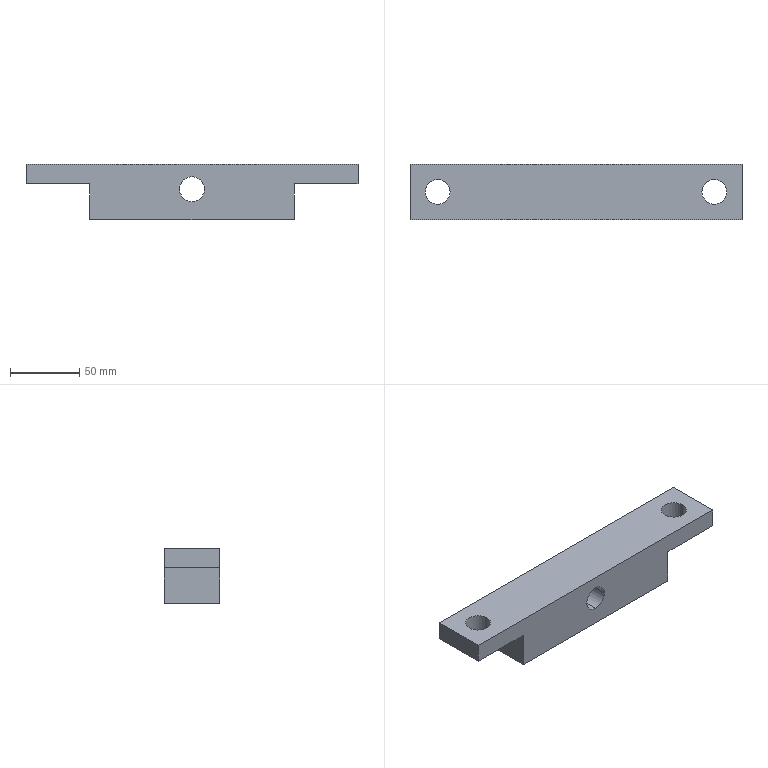Part | SolidWorks | features BaseBody 1 | 1 solid | 16 faces | box 240 x 40 x 40 mm | volume 271016 mm3 | plane 10 | cylinder 6 | commonest cylinder face diameters 18 x6
STEP:
#1=CARTESIAN_POINT('',(91.,0.,6.));
#2=VERTEX_POINT('',#1);
#3=CARTESIAN_POINT('',(109.,0.,6.));
#4=VERTEX_POINT('',#3);
#5=CARTESIAN_POINT('',(100.,0.,6.));
#6=DIRECTION('',(0.,0.,1.));
#7=DIRECTION('',(1.,0.,0.));
#8=AXIS2_PLACEMENT_3D('',#5,#6,#7);
#9=CIRCLE('',#8,9.);
#10=EDGE_CURVE('',#2,#4,#9,.T.);
#11=ORIENTED_EDGE('',*,*,#10,.F.);
#12=CARTESIAN_POINT('',(91.,0.,20.));
#13=VERTEX_POINT('',#12);
#14=CARTESIAN_POINT('',(91.,0.,-20.));
#15=DIRECTION('',(0.,0.,1.));
#16=VECTOR('',#15,1000.);
#17=LINE('',#14,#16);
#18=EDGE_CURVE('',#2,#13,#17,.T.);
#19=ORIENTED_EDGE('',*,*,#18,.T.);
#20=CARTESIAN_POINT('',(109.,0.,20.));
#21=VERTEX_POINT('',#20);
#22=CARTESIAN_POINT('',(100.,0.,20.));
#23=DIRECTION('',(0.,0.,1.));
#24=DIRECTION('',(-1.,0.,0.));
#25=AXIS2_PLACEMENT_3D('',#22,#23,#24);
#26=CIRCLE('',#25,9.);
#27=EDGE_CURVE('',#13,#21,#26,.T.);
#28=ORIENTED_EDGE('',*,*,#27,.T.);
#29=CARTESIAN_POINT('',(109.,0.,-20.));
#30=DIRECTION('',(0.,0.,1.));
#31=VECTOR('',#30,1000.);
#32=LINE('',#29,#31);
#33=EDGE_CURVE('',#4,#21,#32,.T.);
#34=ORIENTED_EDGE('',*,*,#33,.F.);
#35=EDGE_LOOP('',(#11,#19,#28,#34));
#36=FACE_OUTER_BOUND('',#35,.T.);
#37=CARTESIAN_POINT('',(100.,0.,-20.));
#38=DIRECTION('',(0.,0.,1.));
#39=DIRECTION('',(1.,0.,0.));
#40=AXIS2_PLACEMENT_3D('',#37,#38,#39);
#41=CYLINDRICAL_SURFACE('',#40,9.);
#42=ADVANCED_FACE('',(#36),#41,.F.);
#43=CARTESIAN_POINT('',(-109.,0.,6.));
#44=VERTEX_POINT('',#43);
#45=CARTESIAN_POINT('',(-91.,0.,6.));
#46=VERTEX_POINT('',#45);
#47=CARTESIAN_POINT('',(-100.,0.,6.));
#48=DIRECTION('',(0.,0.,1.));
#49=DIRECTION('',(1.,0.,0.));
#50=AXIS2_PLACEMENT_3D('',#47,#48,#49);
#51=CIRCLE('',#50,9.);
#52=EDGE_CURVE('',#44,#46,#51,.T.);
#53=ORIENTED_EDGE('',*,*,#52,.F.);
#54=CARTESIAN_POINT('',(-109.,0.,20.));
#55=VERTEX_POINT('',#54);
#56=CARTESIAN_POINT('',(-109.,0.,-20.));
#57=DIRECTION('',(0.,0.,1.));
#58=VECTOR('',#57,1000.);
#59=LINE('',#56,#58);
#60=EDGE_CURVE('',#44,#55,#59,.T.);
#61=ORIENTED_EDGE('',*,*,#60,.T.);
#62=CARTESIAN_POINT('',(-91.,0.,20.));
#63=VERTEX_POINT('',#62);
#64=CARTESIAN_POINT('',(-100.,0.,20.));
#65=DIRECTION('',(0.,0.,1.));
#66=DIRECTION('',(1.,0.,0.));
#67=AXIS2_PLACEMENT_3D('',#64,#65,#66);
#68=CIRCLE('',#67,9.);
#69=EDGE_CURVE('',#55,#63,#68,.T.);
#70=ORIENTED_EDGE('',*,*,#69,.T.);
#71=CARTESIAN_POINT('',(-91.,0.,-20.));
#72=DIRECTION('',(0.,0.,1.));
#73=VECTOR('',#72,1000.);
#74=LINE('',#71,#73);
#75=EDGE_CURVE('',#46,#63,#74,.T.);
#76=ORIENTED_EDGE('',*,*,#75,.F.);
#77=EDGE_LOOP('',(#53,#61,#70,#76));
#78=FACE_OUTER_BOUND('',#77,.T.);
#79=CARTESIAN_POINT('',(-100.,0.,-20.));
#80=DIRECTION('',(0.,0.,1.));
#81=DIRECTION('',(1.,0.,0.));
#82=AXIS2_PLACEMENT_3D('',#79,#80,#81);
#83=CYLINDRICAL_SURFACE('',#82,9.);
#84=ADVANCED_FACE('',(#78),#83,.F.);
#85=CARTESIAN_POINT('',(0.,-20.,-7.));
#86=VERTEX_POINT('',#85);
#87=CARTESIAN_POINT('',(0.,-20.,11.));
#88=VERTEX_POINT('',#87);
#89=CARTESIAN_POINT('',(0.,-20.,2.));
#90=DIRECTION('',(0.,1.,0.));
#91=DIRECTION('',(0.,0.,1.));
#92=AXIS2_PLACEMENT_3D('',#89,#90,#91);
#93=CIRCLE('',#92,9.);
#94=EDGE_CURVE('',#86,#88,#93,.T.);
#95=ORIENTED_EDGE('',*,*,#94,.F.);
#96=CARTESIAN_POINT('',(0.,20.,-7.));
#97=VERTEX_POINT('',#96);
#98=CARTESIAN_POINT('',(0.,20.,-7.));
#99=DIRECTION('',(0.,1.,0.));
#100=VECTOR('',#99,1000.);
#101=LINE('',#98,#100);
#102=EDGE_CURVE('',#86,#97,#101,.T.);
#103=ORIENTED_EDGE('',*,*,#102,.T.);
#104=CARTESIAN_POINT('',(0.,20.,11.));
#105=VERTEX_POINT('',#104);
#106=CARTESIAN_POINT('',(0.,20.,2.));
#107=DIRECTION('',(0.,1.,0.));
#108=DIRECTION('',(0.,0.,1.));
#109=AXIS2_PLACEMENT_3D('',#106,#107,#108);
#110=CIRCLE('',#109,9.);
#111=EDGE_CURVE('',#97,#105,#110,.T.);
#112=ORIENTED_EDGE('',*,*,#111,.T.);
#113=CARTESIAN_POINT('',(0.,20.,11.));
#114=DIRECTION('',(0.,1.,0.));
#115=VECTOR('',#114,1000.);
#116=LINE('',#113,#115);
#117=EDGE_CURVE('',#88,#105,#116,.T.);
#118=ORIENTED_EDGE('',*,*,#117,.F.);
#119=EDGE_LOOP('',(#95,#103,#112,#118));
#120=FACE_OUTER_BOUND('',#119,.T.);
#121=CARTESIAN_POINT('',(0.,20.,2.));
#122=DIRECTION('',(0.,1.,0.));
#123=DIRECTION('',(0.,0.,1.));
#124=AXIS2_PLACEMENT_3D('',#121,#122,#123);
#125=CYLINDRICAL_SURFACE('',#124,9.);
#126=ADVANCED_FACE('',(#120),#125,.F.);
#127=CARTESIAN_POINT('',(120.,-20.,20.));
#128=VERTEX_POINT('',#127);
#129=CARTESIAN_POINT('',(120.,-20.,6.));
#130=VERTEX_POINT('',#129);
#131=CARTESIAN_POINT('',(120.,-20.,-20.));
#132=DIRECTION('',(0.,0.,-1.));
#133=VECTOR('',#132,1000.);
#134=LINE('',#131,#133);
#135=EDGE_CURVE('',#128,#130,#134,.T.);
#136=ORIENTED_EDGE('',*,*,#135,.T.);
#137=CARTESIAN_POINT('',(120.,20.,6.));
#138=VERTEX_POINT('',#137);
#139=CARTESIAN_POINT('',(120.,-20.,6.));
#140=DIRECTION('',(0.,1.,0.));
#141=VECTOR('',#140,1000.);
#142=LINE('',#139,#141);
#143=EDGE_CURVE('',#130,#138,#142,.T.);
#144=ORIENTED_EDGE('',*,*,#143,.T.);
#145=CARTESIAN_POINT('',(120.,20.,20.));
#146=VERTEX_POINT('',#145);
#147=CARTESIAN_POINT('',(120.,20.,-20.));
#148=DIRECTION('',(0.,0.,-1.));
#149=VECTOR('',#148,1000.);
#150=LINE('',#147,#149);
#151=EDGE_CURVE('',#146,#138,#150,.T.);
#152=ORIENTED_EDGE('',*,*,#151,.F.);
#153=CARTESIAN_POINT('',(120.,20.,20.));
#154=DIRECTION('',(0.,-1.,0.));
#155=VECTOR('',#154,1000.);
#156=LINE('',#153,#155);
#157=EDGE_CURVE('',#146,#128,#156,.T.);
#158=ORIENTED_EDGE('',*,*,#157,.T.);
#159=EDGE_LOOP('',(#136,#144,#152,#158));
#160=FACE_OUTER_BOUND('',#159,.T.);
#161=CARTESIAN_POINT('',(120.,20.,-20.));
#162=DIRECTION('',(-1.,0.,0.));
#163=DIRECTION('',(0.,0.,1.));
#164=AXIS2_PLACEMENT_3D('',#161,#162,#163);
#165=PLANE('',#164);
#166=ADVANCED_FACE('',(#160),#165,.F.);
#167=CARTESIAN_POINT('',(74.,-20.,-20.));
#168=VERTEX_POINT('',#167);
#169=CARTESIAN_POINT('',(-74.,-20.,-20.));
#170=VERTEX_POINT('',#169);
#171=CARTESIAN_POINT('',(-120.,-20.,-20.));
#172=DIRECTION('',(-1.,0.,0.));
#173=VECTOR('',#172,1000.);
#174=LINE('',#171,#173);
#175=EDGE_CURVE('',#168,#170,#174,.T.);
#176=ORIENTED_EDGE('',*,*,#175,.T.);
#177=CARTESIAN_POINT('',(-74.,20.,-20.));
#178=VERTEX_POINT('',#177);
#179=CARTESIAN_POINT('',(-74.,-20.,-20.));
#180=DIRECTION('',(0.,1.,0.));
#181=VECTOR('',#180,1000.);
#182=LINE('',#179,#181);
#183=EDGE_CURVE('',#170,#178,#182,.T.);
#184=ORIENTED_EDGE('',*,*,#183,.T.);
#185=CARTESIAN_POINT('',(74.,20.,-20.));
#186=VERTEX_POINT('',#185);
#187=CARTESIAN_POINT('',(-120.,20.,-20.));
#188=DIRECTION('',(-1.,0.,0.));
#189=VECTOR('',#188,1000.);
#190=LINE('',#187,#189);
#191=EDGE_CURVE('',#186,#178,#190,.T.);
#192=ORIENTED_EDGE('',*,*,#191,.F.);
#193=CARTESIAN_POINT('',(74.,-20.,-20.));
#194=DIRECTION('',(0.,1.,0.));
#195=VECTOR('',#194,1000.);
#196=LINE('',#193,#195);
#197=EDGE_CURVE('',#168,#186,#196,.T.);
#198=ORIENTED_EDGE('',*,*,#197,.F.);
#199=EDGE_LOOP('',(#176,#184,#192,#198));
#200=FACE_OUTER_BOUND('',#199,.T.);
#201=CARTESIAN_POINT('',(-120.,20.,-20.));
#202=DIRECTION('',(0.,0.,1.));
#203=DIRECTION('',(1.,0.,0.));
#204=AXIS2_PLACEMENT_3D('',#201,#202,#203);
#205=PLANE('',#204);
#206=ADVANCED_FACE('',(#200),#205,.F.);
#207=CARTESIAN_POINT('',(-120.,20.,6.));
#208=VERTEX_POINT('',#207);
#209=CARTESIAN_POINT('',(-120.,20.,20.));
#210=VERTEX_POINT('',#209);
#211=CARTESIAN_POINT('',(-120.,20.,-20.));
#212=DIRECTION('',(0.,0.,1.));
#213=VECTOR('',#212,1000.);
#214=LINE('',#211,#213);
#215=EDGE_CURVE('',#208,#210,#214,.T.);
#216=ORIENTED_EDGE('',*,*,#215,.F.);
#217=CARTESIAN_POINT('',(-120.,-20.,6.));
#218=VERTEX_POINT('',#217);
#219=CARTESIAN_POINT('',(-120.,-20.,6.));
#220=DIRECTION('',(0.,1.,0.));
#221=VECTOR('',#220,1000.);
#222=LINE('',#219,#221);
#223=EDGE_CURVE('',#218,#208,#222,.T.);
#224=ORIENTED_EDGE('',*,*,#223,.F.);
#225=CARTESIAN_POINT('',(-120.,-20.,20.));
#226=VERTEX_POINT('',#225);
#227=CARTESIAN_POINT('',(-120.,-20.,-20.));
#228=DIRECTION('',(0.,0.,1.));
#229=VECTOR('',#228,1000.);
#230=LINE('',#227,#229);
#231=EDGE_CURVE('',#218,#226,#230,.T.);
#232=ORIENTED_EDGE('',*,*,#231,.T.);
#233=CARTESIAN_POINT('',(-120.,20.,20.));
#234=DIRECTION('',(0.,-1.,0.));
#235=VECTOR('',#234,1000.);
#236=LINE('',#233,#235);
#237=EDGE_CURVE('',#210,#226,#236,.T.);
#238=ORIENTED_EDGE('',*,*,#237,.F.);
#239=EDGE_LOOP('',(#216,#224,#232,#238));
#240=FACE_OUTER_BOUND('',#239,.T.);
#241=CARTESIAN_POINT('',(-120.,20.,-20.));
#242=DIRECTION('',(1.,0.,0.));
#243=DIRECTION('',(0.,0.,-1.));
#244=AXIS2_PLACEMENT_3D('',#241,#242,#243);
#245=PLANE('',#244);
#246=ADVANCED_FACE('',(#240),#245,.F.);
#247=CARTESIAN_POINT('',(-100.,0.,20.));
#248=DIRECTION('',(0.,0.,1.));
#249=DIRECTION('',(1.,0.,0.));
#250=AXIS2_PLACEMENT_3D('',#247,#248,#249);
#251=CIRCLE('',#250,9.);
#252=EDGE_CURVE('',#63,#55,#251,.T.);
#253=ORIENTED_EDGE('',*,*,#252,.F.);
#254=ORIENTED_EDGE('',*,*,#69,.F.);
#255=EDGE_LOOP('',(#253,#254));
#256=FACE_BOUND('',#255,.T.);
#257=CARTESIAN_POINT('',(100.,0.,20.));
#258=DIRECTION('',(0.,0.,1.));
#259=DIRECTION('',(-1.,0.,0.));
#260=AXIS2_PLACEMENT_3D('',#257,#258,#259);
#261=CIRCLE('',#260,9.);
#262=EDGE_CURVE('',#21,#13,#261,.T.);
#263=ORIENTED_EDGE('',*,*,#262,.F.);
#264=ORIENTED_EDGE('',*,*,#27,.F.);
#265=EDGE_LOOP('',(#263,#264));
#266=FACE_BOUND('',#265,.T.);
#267=CARTESIAN_POINT('',(-120.,-20.,20.));
#268=DIRECTION('',(1.,0.,0.));
#269=VECTOR('',#268,1000.);
#270=LINE('',#267,#269);
#271=EDGE_CURVE('',#226,#128,#270,.T.);
#272=ORIENTED_EDGE('',*,*,#271,.T.);
#273=ORIENTED_EDGE('',*,*,#157,.F.);
#274=CARTESIAN_POINT('',(-120.,20.,20.));
#275=DIRECTION('',(1.,0.,0.));
#276=VECTOR('',#275,1000.);
#277=LINE('',#274,#276);
#278=EDGE_CURVE('',#210,#146,#277,.T.);
#279=ORIENTED_EDGE('',*,*,#278,.F.);
#280=ORIENTED_EDGE('',*,*,#237,.T.);
#281=EDGE_LOOP('',(#272,#273,#279,#280));
#282=FACE_OUTER_BOUND('',#281,.T.);
#283=CARTESIAN_POINT('',(-120.,20.,20.));
#284=DIRECTION('',(0.,0.,-1.));
#285=DIRECTION('',(-1.,0.,0.));
#286=AXIS2_PLACEMENT_3D('',#283,#284,#285);
#287=PLANE('',#286);
#288=ADVANCED_FACE('',(#256,#266,#282),#287,.F.);
#289=CARTESIAN_POINT('',(0.,20.,2.));
#290=DIRECTION('',(0.,1.,0.));
#291=DIRECTION('',(0.,0.,1.));
#292=AXIS2_PLACEMENT_3D('',#289,#290,#291);
#293=CIRCLE('',#292,9.);
#294=EDGE_CURVE('',#105,#97,#293,.T.);
#295=ORIENTED_EDGE('',*,*,#294,.F.);
#296=ORIENTED_EDGE('',*,*,#111,.F.);
#297=EDGE_LOOP('',(#295,#296));
#298=FACE_BOUND('',#297,.T.);
#299=CARTESIAN_POINT('',(-74.,20.,6.));
#300=VERTEX_POINT('',#299);
#301=CARTESIAN_POINT('',(-74.,20.,-20.));
#302=DIRECTION('',(0.,0.,-1.));
#303=VECTOR('',#302,1000.);
#304=LINE('',#301,#303);
#305=EDGE_CURVE('',#300,#178,#304,.T.);
#306=ORIENTED_EDGE('',*,*,#305,.F.);
#307=CARTESIAN_POINT('',(-120.,20.,6.));
#308=DIRECTION('',(1.,0.,0.));
#309=VECTOR('',#308,1000.);
#310=LINE('',#307,#309);
#311=EDGE_CURVE('',#208,#300,#310,.T.);
#312=ORIENTED_EDGE('',*,*,#311,.F.);
#313=ORIENTED_EDGE('',*,*,#215,.T.);
#314=ORIENTED_EDGE('',*,*,#278,.T.);
#315=ORIENTED_EDGE('',*,*,#151,.T.);
#316=CARTESIAN_POINT('',(74.,20.,6.));
#317=VERTEX_POINT('',#316);
#318=CARTESIAN_POINT('',(120.,20.,6.));
#319=DIRECTION('',(1.,0.,0.));
#320=VECTOR('',#319,1000.);
#321=LINE('',#318,#320);
#322=EDGE_CURVE('',#317,#138,#321,.T.);
#323=ORIENTED_EDGE('',*,*,#322,.F.);
#324=CARTESIAN_POINT('',(74.,20.,-20.));
#325=DIRECTION('',(0.,0.,1.));
#326=VECTOR('',#325,1000.);
#327=LINE('',#324,#326);
#328=EDGE_CURVE('',#186,#317,#327,.T.);
#329=ORIENTED_EDGE('',*,*,#328,.F.);
#330=ORIENTED_EDGE('',*,*,#191,.T.);
#331=EDGE_LOOP('',(#306,#312,#313,#314,#315,#323,#329,#330));
#332=FACE_OUTER_BOUND('',#331,.T.);
#333=CARTESIAN_POINT('',(0.,20.,0.));
#334=DIRECTION('',(0.,1.,0.));
#335=DIRECTION('',(0.,0.,1.));
#336=AXIS2_PLACEMENT_3D('',#333,#334,#335);
#337=PLANE('',#336);
#338=ADVANCED_FACE('',(#298,#332),#337,.T.);
#339=CARTESIAN_POINT('',(0.,-20.,2.));
#340=DIRECTION('',(0.,1.,0.));
#341=DIRECTION('',(0.,0.,1.));
#342=AXIS2_PLACEMENT_3D('',#339,#340,#341);
#343=CIRCLE('',#342,9.);
#344=EDGE_CURVE('',#88,#86,#343,.T.);
#345=ORIENTED_EDGE('',*,*,#344,.T.);
#346=ORIENTED_EDGE('',*,*,#94,.T.);
#347=EDGE_LOOP('',(#345,#346));
#348=FACE_BOUND('',#347,.T.);
#349=CARTESIAN_POINT('',(-74.,-20.,6.));
#350=VERTEX_POINT('',#349);
#351=CARTESIAN_POINT('',(-120.,-20.,6.));
#352=DIRECTION('',(1.,0.,0.));
#353=VECTOR('',#352,1000.);
#354=LINE('',#351,#353);
#355=EDGE_CURVE('',#218,#350,#354,.T.);
#356=ORIENTED_EDGE('',*,*,#355,.T.);
#357=CARTESIAN_POINT('',(-74.,-20.,-20.));
#358=DIRECTION('',(0.,0.,-1.));
#359=VECTOR('',#358,1000.);
#360=LINE('',#357,#359);
#361=EDGE_CURVE('',#350,#170,#360,.T.);
#362=ORIENTED_EDGE('',*,*,#361,.T.);
#363=ORIENTED_EDGE('',*,*,#175,.F.);
#364=CARTESIAN_POINT('',(74.,-20.,6.));
#365=VERTEX_POINT('',#364);
#366=CARTESIAN_POINT('',(74.,-20.,-20.));
#367=DIRECTION('',(0.,0.,1.));
#368=VECTOR('',#367,1000.);
#369=LINE('',#366,#368);
#370=EDGE_CURVE('',#168,#365,#369,.T.);
#371=ORIENTED_EDGE('',*,*,#370,.T.);
#372=CARTESIAN_POINT('',(120.,-20.,6.));
#373=DIRECTION('',(1.,0.,0.));
#374=VECTOR('',#373,1000.);
#375=LINE('',#372,#374);
#376=EDGE_CURVE('',#365,#130,#375,.T.);
#377=ORIENTED_EDGE('',*,*,#376,.T.);
#378=ORIENTED_EDGE('',*,*,#135,.F.);
#379=ORIENTED_EDGE('',*,*,#271,.F.);
#380=ORIENTED_EDGE('',*,*,#231,.F.);
#381=EDGE_LOOP('',(#356,#362,#363,#371,#377,#378,#379,#380));
#382=FACE_OUTER_BOUND('',#381,.T.);
#383=CARTESIAN_POINT('',(0.,-20.,0.));
#384=DIRECTION('',(0.,1.,0.));
#385=DIRECTION('',(0.,0.,1.));
#386=AXIS2_PLACEMENT_3D('',#383,#384,#385);
#387=PLANE('',#386);
#388=ADVANCED_FACE('',(#348,#382),#387,.F.);
#389=CARTESIAN_POINT('',(100.,0.,6.));
#390=DIRECTION('',(0.,0.,1.));
#391=DIRECTION('',(1.,0.,0.));
#392=AXIS2_PLACEMENT_3D('',#389,#390,#391);
#393=CIRCLE('',#392,9.);
#394=EDGE_CURVE('',#4,#2,#393,.T.);
#395=ORIENTED_EDGE('',*,*,#394,.T.);
#396=ORIENTED_EDGE('',*,*,#10,.T.);
#397=EDGE_LOOP('',(#395,#396));
#398=FACE_BOUND('',#397,.T.);
#399=ORIENTED_EDGE('',*,*,#322,.T.);
#400=ORIENTED_EDGE('',*,*,#143,.F.);
#401=ORIENTED_EDGE('',*,*,#376,.F.);
#402=CARTESIAN_POINT('',(74.,-20.,6.));
#403=DIRECTION('',(0.,1.,0.));
#404=VECTOR('',#403,1000.);
#405=LINE('',#402,#404);
#406=EDGE_CURVE('',#365,#317,#405,.T.);
#407=ORIENTED_EDGE('',*,*,#406,.T.);
#408=EDGE_LOOP('',(#399,#400,#401,#407));
#409=FACE_OUTER_BOUND('',#408,.T.);
#410=CARTESIAN_POINT('',(120.,-20.,6.));
#411=DIRECTION('',(0.,0.,1.));
#412=DIRECTION('',(1.,0.,0.));
#413=AXIS2_PLACEMENT_3D('',#410,#411,#412);
#414=PLANE('',#413);
#415=ADVANCED_FACE('',(#398,#409),#414,.F.);
#416=ORIENTED_EDGE('',*,*,#328,.T.);
#417=ORIENTED_EDGE('',*,*,#406,.F.);
#418=ORIENTED_EDGE('',*,*,#370,.F.);
#419=ORIENTED_EDGE('',*,*,#197,.T.);
#420=EDGE_LOOP('',(#416,#417,#418,#419));
#421=FACE_OUTER_BOUND('',#420,.T.);
#422=CARTESIAN_POINT('',(74.,-20.,-20.));
#423=DIRECTION('',(-1.,0.,0.));
#424=DIRECTION('',(0.,0.,1.));
#425=AXIS2_PLACEMENT_3D('',#422,#423,#424);
#426=PLANE('',#425);
#427=ADVANCED_FACE('',(#421),#426,.F.);
#428=ORIENTED_EDGE('',*,*,#305,.T.);
#429=ORIENTED_EDGE('',*,*,#183,.F.);
#430=ORIENTED_EDGE('',*,*,#361,.F.);
#431=CARTESIAN_POINT('',(-74.,-20.,6.));
#432=DIRECTION('',(0.,1.,0.));
#433=VECTOR('',#432,1000.);
#434=LINE('',#431,#433);
#435=EDGE_CURVE('',#350,#300,#434,.T.);
#436=ORIENTED_EDGE('',*,*,#435,.T.);
#437=EDGE_LOOP('',(#428,#429,#430,#436));
#438=FACE_OUTER_BOUND('',#437,.T.);
#439=CARTESIAN_POINT('',(-74.,-20.,-20.));
#440=DIRECTION('',(1.,0.,0.));
#441=DIRECTION('',(0.,0.,-1.));
#442=AXIS2_PLACEMENT_3D('',#439,#440,#441);
#443=PLANE('',#442);
#444=ADVANCED_FACE('',(#438),#443,.F.);
#445=CARTESIAN_POINT('',(-100.,0.,6.));
#446=DIRECTION('',(0.,0.,1.));
#447=DIRECTION('',(1.,0.,0.));
#448=AXIS2_PLACEMENT_3D('',#445,#446,#447);
#449=CIRCLE('',#448,9.);
#450=EDGE_CURVE('',#46,#44,#449,.T.);
#451=ORIENTED_EDGE('',*,*,#450,.T.);
#452=ORIENTED_EDGE('',*,*,#52,.T.);
#453=EDGE_LOOP('',(#451,#452));
#454=FACE_BOUND('',#453,.T.);
#455=ORIENTED_EDGE('',*,*,#311,.T.);
#456=ORIENTED_EDGE('',*,*,#435,.F.);
#457=ORIENTED_EDGE('',*,*,#355,.F.);
#458=ORIENTED_EDGE('',*,*,#223,.T.);
#459=EDGE_LOOP('',(#455,#456,#457,#458));
#460=FACE_OUTER_BOUND('',#459,.T.);
#461=CARTESIAN_POINT('',(-120.,-20.,6.));
#462=DIRECTION('',(0.,0.,1.));
#463=DIRECTION('',(1.,0.,0.));
#464=AXIS2_PLACEMENT_3D('',#461,#462,#463);
#465=PLANE('',#464);
#466=ADVANCED_FACE('',(#454,#460),#465,.F.);
#467=ORIENTED_EDGE('',*,*,#102,.F.);
#468=ORIENTED_EDGE('',*,*,#344,.F.);
#469=ORIENTED_EDGE('',*,*,#117,.T.);
#470=ORIENTED_EDGE('',*,*,#294,.T.);
#471=EDGE_LOOP('',(#467,#468,#469,#470));
#472=FACE_OUTER_BOUND('',#471,.T.);
#473=CARTESIAN_POINT('',(0.,20.,2.));
#474=DIRECTION('',(0.,1.,0.));
#475=DIRECTION('',(0.,0.,1.));
#476=AXIS2_PLACEMENT_3D('',#473,#474,#475);
#477=CYLINDRICAL_SURFACE('',#476,9.);
#478=ADVANCED_FACE('',(#472),#477,.F.);
#479=ORIENTED_EDGE('',*,*,#60,.F.);
#480=ORIENTED_EDGE('',*,*,#450,.F.);
#481=ORIENTED_EDGE('',*,*,#75,.T.);
#482=ORIENTED_EDGE('',*,*,#252,.T.);
#483=EDGE_LOOP('',(#479,#480,#481,#482));
#484=FACE_OUTER_BOUND('',#483,.T.);
#485=CARTESIAN_POINT('',(-100.,0.,-20.));
#486=DIRECTION('',(0.,0.,1.));
#487=DIRECTION('',(1.,0.,0.));
#488=AXIS2_PLACEMENT_3D('',#485,#486,#487);
#489=CYLINDRICAL_SURFACE('',#488,9.);
#490=ADVANCED_FACE('',(#484),#489,.F.);
#491=ORIENTED_EDGE('',*,*,#18,.F.);
#492=ORIENTED_EDGE('',*,*,#394,.F.);
#493=ORIENTED_EDGE('',*,*,#33,.T.);
#494=ORIENTED_EDGE('',*,*,#262,.T.);
#495=EDGE_LOOP('',(#491,#492,#493,#494));
#496=FACE_OUTER_BOUND('',#495,.T.);
#497=CARTESIAN_POINT('',(100.,0.,-20.));
#498=DIRECTION('',(0.,0.,1.));
#499=DIRECTION('',(1.,0.,0.));
#500=AXIS2_PLACEMENT_3D('',#497,#498,#499);
#501=CYLINDRICAL_SURFACE('',#500,9.);
#502=ADVANCED_FACE('',(#496),#501,.F.);
#503=CLOSED_SHELL('',(#42,#84,#126,#166,#206,#246,#288,#338,#388,#415,#427,#444,#466,#478,#490,#502));
#504=MANIFOLD_SOLID_BREP('',#503);
#505=CARTESIAN_POINT('',(0.,0.,0.));
#506=DIRECTION('',(0.,0.,1.));
#507=DIRECTION('',(1.,0.,0.));
#508=AXIS2_PLACEMENT_3D('',#505,#506,#507);
#509=(LENGTH_UNIT()NAMED_UNIT(*)SI_UNIT(.MILLI.,.METRE.));
#510=UNCERTAINTY_MEASURE_WITH_UNIT(LENGTH_MEASURE(0.00001),#509,'','');
#511=(NAMED_UNIT(*)PLANE_ANGLE_UNIT()SI_UNIT($,.RADIAN.));
#512=(NAMED_UNIT(*)SI_UNIT($,.STERADIAN.)SOLID_ANGLE_UNIT());
#513=(GEOMETRIC_REPRESENTATION_CONTEXT(3)GLOBAL_UNCERTAINTY_ASSIGNED_CONTEXT((#510))GLOBAL_UNIT_ASSIGNED_CONTEXT((#509,#511,#512))REPRESENTATION_CONTEXT('',''));
#514=ADVANCED_BREP_SHAPE_REPRESENTATION('',(#504,#508),#513);